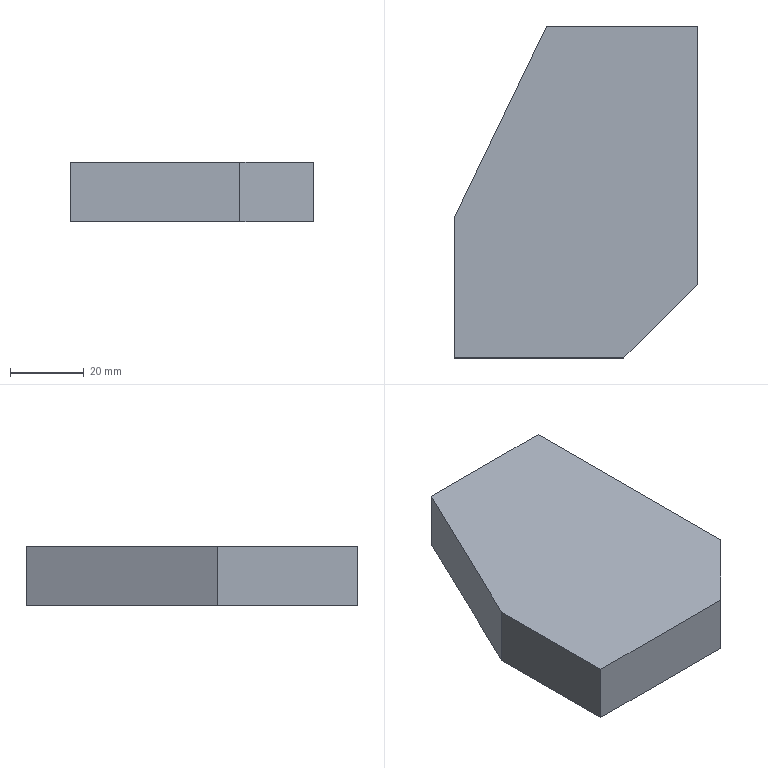Part | SolidWorks | features Chamfer 1, Extrusion 1 | 1 solid | 8 faces | box 66 x 90 x 16 mm | volume 81440 mm3 | plane 8
STEP:
#1=CARTESIAN_POINT('',(0.,38.,-8.));
#2=VERTEX_POINT('',#1);
#3=CARTESIAN_POINT('',(0.,0.,-8.));
#4=VERTEX_POINT('',#3);
#5=CARTESIAN_POINT('',(0.,0.,-8.));
#6=DIRECTION('',(0.,-1.,0.));
#7=VECTOR('',#6,1000.);
#8=LINE('',#5,#7);
#9=EDGE_CURVE('',#2,#4,#8,.T.);
#10=ORIENTED_EDGE('',*,*,#9,.T.);
#11=CARTESIAN_POINT('',(0.,0.,8.));
#12=VERTEX_POINT('',#11);
#13=CARTESIAN_POINT('',(0.,0.,8.));
#14=DIRECTION('',(0.,0.,-1.));
#15=VECTOR('',#14,1000.);
#16=LINE('',#13,#15);
#17=EDGE_CURVE('',#12,#4,#16,.T.);
#18=ORIENTED_EDGE('',*,*,#17,.F.);
#19=CARTESIAN_POINT('',(0.,38.,8.));
#20=VERTEX_POINT('',#19);
#21=CARTESIAN_POINT('',(0.,0.,8.));
#22=DIRECTION('',(0.,-1.,0.));
#23=VECTOR('',#22,1000.);
#24=LINE('',#21,#23);
#25=EDGE_CURVE('',#20,#12,#24,.T.);
#26=ORIENTED_EDGE('',*,*,#25,.F.);
#27=CARTESIAN_POINT('',(0.,38.,8.));
#28=DIRECTION('',(0.,0.,-1.));
#29=VECTOR('',#28,1000.);
#30=LINE('',#27,#29);
#31=EDGE_CURVE('',#20,#2,#30,.T.);
#32=ORIENTED_EDGE('',*,*,#31,.T.);
#33=EDGE_LOOP('',(#10,#18,#26,#32));
#34=FACE_OUTER_BOUND('',#33,.T.);
#35=CARTESIAN_POINT('',(0.,0.,8.));
#36=DIRECTION('',(1.,0.,0.));
#37=DIRECTION('',(0.,0.,-1.));
#38=AXIS2_PLACEMENT_3D('',#35,#36,#37);
#39=PLANE('',#38);
#40=ADVANCED_FACE('',(#34),#39,.F.);
#41=CARTESIAN_POINT('',(46.,0.,-8.));
#42=VERTEX_POINT('',#41);
#43=CARTESIAN_POINT('',(66.,0.,-8.));
#44=DIRECTION('',(1.,0.,0.));
#45=VECTOR('',#44,1000.);
#46=LINE('',#43,#45);
#47=EDGE_CURVE('',#4,#42,#46,.T.);
#48=ORIENTED_EDGE('',*,*,#47,.T.);
#49=CARTESIAN_POINT('',(46.,0.,8.));
#50=VERTEX_POINT('',#49);
#51=CARTESIAN_POINT('',(46.,0.,8.));
#52=DIRECTION('',(0.,0.,1.));
#53=VECTOR('',#52,1000.);
#54=LINE('',#51,#53);
#55=EDGE_CURVE('',#42,#50,#54,.T.);
#56=ORIENTED_EDGE('',*,*,#55,.T.);
#57=CARTESIAN_POINT('',(66.,0.,8.));
#58=DIRECTION('',(1.,0.,0.));
#59=VECTOR('',#58,1000.);
#60=LINE('',#57,#59);
#61=EDGE_CURVE('',#12,#50,#60,.T.);
#62=ORIENTED_EDGE('',*,*,#61,.F.);
#63=ORIENTED_EDGE('',*,*,#17,.T.);
#64=EDGE_LOOP('',(#48,#56,#62,#63));
#65=FACE_OUTER_BOUND('',#64,.T.);
#66=CARTESIAN_POINT('',(66.,0.,8.));
#67=DIRECTION('',(0.,1.,0.));
#68=DIRECTION('',(-1.,0.,0.));
#69=AXIS2_PLACEMENT_3D('',#66,#67,#68);
#70=PLANE('',#69);
#71=ADVANCED_FACE('',(#65),#70,.F.);
#72=CARTESIAN_POINT('',(66.,20.,8.));
#73=VERTEX_POINT('',#72);
#74=CARTESIAN_POINT('',(66.,90.,8.));
#75=VERTEX_POINT('',#74);
#76=CARTESIAN_POINT('',(66.,90.,8.));
#77=DIRECTION('',(0.,1.,0.));
#78=VECTOR('',#77,1000.);
#79=LINE('',#76,#78);
#80=EDGE_CURVE('',#73,#75,#79,.T.);
#81=ORIENTED_EDGE('',*,*,#80,.F.);
#82=CARTESIAN_POINT('',(66.,20.,-8.));
#83=VERTEX_POINT('',#82);
#84=CARTESIAN_POINT('',(66.,20.,8.));
#85=DIRECTION('',(0.,0.,-1.));
#86=VECTOR('',#85,1000.);
#87=LINE('',#84,#86);
#88=EDGE_CURVE('',#73,#83,#87,.T.);
#89=ORIENTED_EDGE('',*,*,#88,.T.);
#90=CARTESIAN_POINT('',(66.,90.,-8.));
#91=VERTEX_POINT('',#90);
#92=CARTESIAN_POINT('',(66.,90.,-8.));
#93=DIRECTION('',(0.,1.,0.));
#94=VECTOR('',#93,1000.);
#95=LINE('',#92,#94);
#96=EDGE_CURVE('',#83,#91,#95,.T.);
#97=ORIENTED_EDGE('',*,*,#96,.T.);
#98=CARTESIAN_POINT('',(66.,90.,8.));
#99=DIRECTION('',(0.,0.,-1.));
#100=VECTOR('',#99,1000.);
#101=LINE('',#98,#100);
#102=EDGE_CURVE('',#75,#91,#101,.T.);
#103=ORIENTED_EDGE('',*,*,#102,.F.);
#104=EDGE_LOOP('',(#81,#89,#97,#103));
#105=FACE_OUTER_BOUND('',#104,.T.);
#106=CARTESIAN_POINT('',(66.,90.,8.));
#107=DIRECTION('',(-1.,0.,0.));
#108=DIRECTION('',(0.,-1.,0.));
#109=AXIS2_PLACEMENT_3D('',#106,#107,#108);
#110=PLANE('',#109);
#111=ADVANCED_FACE('',(#105),#110,.F.);
#112=CARTESIAN_POINT('',(25.,90.,-8.));
#113=VERTEX_POINT('',#112);
#114=CARTESIAN_POINT('',(25.,90.,-8.));
#115=DIRECTION('',(-1.,0.,0.));
#116=VECTOR('',#115,1000.);
#117=LINE('',#114,#116);
#118=EDGE_CURVE('',#91,#113,#117,.T.);
#119=ORIENTED_EDGE('',*,*,#118,.T.);
#120=CARTESIAN_POINT('',(25.,90.,8.));
#121=VERTEX_POINT('',#120);
#122=CARTESIAN_POINT('',(25.,90.,8.));
#123=DIRECTION('',(0.,0.,-1.));
#124=VECTOR('',#123,1000.);
#125=LINE('',#122,#124);
#126=EDGE_CURVE('',#121,#113,#125,.T.);
#127=ORIENTED_EDGE('',*,*,#126,.F.);
#128=CARTESIAN_POINT('',(25.,90.,8.));
#129=DIRECTION('',(-1.,0.,0.));
#130=VECTOR('',#129,1000.);
#131=LINE('',#128,#130);
#132=EDGE_CURVE('',#75,#121,#131,.T.);
#133=ORIENTED_EDGE('',*,*,#132,.F.);
#134=ORIENTED_EDGE('',*,*,#102,.T.);
#135=EDGE_LOOP('',(#119,#127,#133,#134));
#136=FACE_OUTER_BOUND('',#135,.T.);
#137=CARTESIAN_POINT('',(25.,90.,8.));
#138=DIRECTION('',(0.,-1.,0.));
#139=DIRECTION('',(0.,0.,-1.));
#140=AXIS2_PLACEMENT_3D('',#137,#138,#139);
#141=PLANE('',#140);
#142=ADVANCED_FACE('',(#136),#141,.F.);
#143=CARTESIAN_POINT('',(0.,38.,-8.));
#144=DIRECTION('',(-0.4333,-0.9013,0.));
#145=VECTOR('',#144,1000.);
#146=LINE('',#143,#145);
#147=EDGE_CURVE('',#113,#2,#146,.T.);
#148=ORIENTED_EDGE('',*,*,#147,.T.);
#149=ORIENTED_EDGE('',*,*,#31,.F.);
#150=CARTESIAN_POINT('',(0.,38.,8.));
#151=DIRECTION('',(-0.4333,-0.9013,0.));
#152=VECTOR('',#151,1000.);
#153=LINE('',#150,#152);
#154=EDGE_CURVE('',#121,#20,#153,.T.);
#155=ORIENTED_EDGE('',*,*,#154,.F.);
#156=ORIENTED_EDGE('',*,*,#126,.T.);
#157=EDGE_LOOP('',(#148,#149,#155,#156));
#158=FACE_OUTER_BOUND('',#157,.T.);
#159=CARTESIAN_POINT('',(0.,38.,8.));
#160=DIRECTION('',(0.9013,-0.4333,0.));
#161=DIRECTION('',(0.4333,0.9013,0.));
#162=AXIS2_PLACEMENT_3D('',#159,#160,#161);
#163=PLANE('',#162);
#164=ADVANCED_FACE('',(#158),#163,.F.);
#165=ORIENTED_EDGE('',*,*,#61,.T.);
#166=CARTESIAN_POINT('',(66.,20.,8.));
#167=DIRECTION('',(0.7071,0.7071,0.));
#168=VECTOR('',#167,1000.);
#169=LINE('',#166,#168);
#170=EDGE_CURVE('',#50,#73,#169,.T.);
#171=ORIENTED_EDGE('',*,*,#170,.T.);
#172=ORIENTED_EDGE('',*,*,#80,.T.);
#173=ORIENTED_EDGE('',*,*,#132,.T.);
#174=ORIENTED_EDGE('',*,*,#154,.T.);
#175=ORIENTED_EDGE('',*,*,#25,.T.);
#176=EDGE_LOOP('',(#165,#171,#172,#173,#174,#175));
#177=FACE_OUTER_BOUND('',#176,.T.);
#178=CARTESIAN_POINT('',(0.,0.,8.));
#179=DIRECTION('',(0.,0.,-1.));
#180=DIRECTION('',(-1.,0.,0.));
#181=AXIS2_PLACEMENT_3D('',#178,#179,#180);
#182=PLANE('',#181);
#183=ADVANCED_FACE('',(#177),#182,.F.);
#184=ORIENTED_EDGE('',*,*,#96,.F.);
#185=CARTESIAN_POINT('',(23.,-23.,-8.));
#186=DIRECTION('',(-0.7071,-0.7071,0.));
#187=VECTOR('',#186,1000.);
#188=LINE('',#185,#187);
#189=EDGE_CURVE('',#83,#42,#188,.T.);
#190=ORIENTED_EDGE('',*,*,#189,.T.);
#191=ORIENTED_EDGE('',*,*,#47,.F.);
#192=ORIENTED_EDGE('',*,*,#9,.F.);
#193=ORIENTED_EDGE('',*,*,#147,.F.);
#194=ORIENTED_EDGE('',*,*,#118,.F.);
#195=EDGE_LOOP('',(#184,#190,#191,#192,#193,#194));
#196=FACE_OUTER_BOUND('',#195,.T.);
#197=CARTESIAN_POINT('',(0.,0.,-8.));
#198=DIRECTION('',(0.,0.,-1.));
#199=DIRECTION('',(-1.,0.,0.));
#200=AXIS2_PLACEMENT_3D('',#197,#198,#199);
#201=PLANE('',#200);
#202=ADVANCED_FACE('',(#196),#201,.T.);
#203=ORIENTED_EDGE('',*,*,#170,.F.);
#204=ORIENTED_EDGE('',*,*,#55,.F.);
#205=ORIENTED_EDGE('',*,*,#189,.F.);
#206=ORIENTED_EDGE('',*,*,#88,.F.);
#207=EDGE_LOOP('',(#203,#204,#205,#206));
#208=FACE_OUTER_BOUND('',#207,.T.);
#209=CARTESIAN_POINT('',(66.,20.,8.));
#210=DIRECTION('',(-0.7071,0.7071,0.));
#211=DIRECTION('',(0.,0.,-1.));
#212=AXIS2_PLACEMENT_3D('',#209,#210,#211);
#213=PLANE('',#212);
#214=ADVANCED_FACE('',(#208),#213,.F.);
#215=CLOSED_SHELL('',(#40,#71,#111,#142,#164,#183,#202,#214));
#216=MANIFOLD_SOLID_BREP('',#215);
#217=CARTESIAN_POINT('',(0.,0.,0.));
#218=DIRECTION('',(0.,0.,1.));
#219=DIRECTION('',(1.,0.,0.));
#220=AXIS2_PLACEMENT_3D('',#217,#218,#219);
#221=(LENGTH_UNIT()NAMED_UNIT(*)SI_UNIT(.MILLI.,.METRE.));
#222=UNCERTAINTY_MEASURE_WITH_UNIT(LENGTH_MEASURE(0.00001),#221,'','');
#223=(NAMED_UNIT(*)PLANE_ANGLE_UNIT()SI_UNIT($,.RADIAN.));
#224=(NAMED_UNIT(*)SI_UNIT($,.STERADIAN.)SOLID_ANGLE_UNIT());
#225=(GEOMETRIC_REPRESENTATION_CONTEXT(3)GLOBAL_UNCERTAINTY_ASSIGNED_CONTEXT((#222))GLOBAL_UNIT_ASSIGNED_CONTEXT((#221,#223,#224))REPRESENTATION_CONTEXT('',''));
#226=ADVANCED_BREP_SHAPE_REPRESENTATION('',(#216,#220),#225);